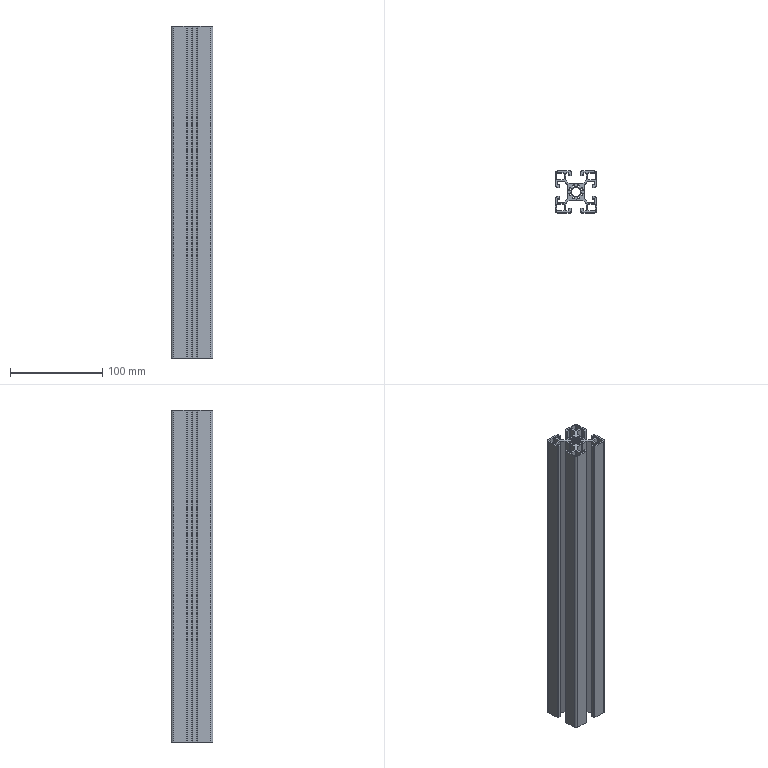Part | STEP file | PN_0029 | 1 solid | 271 faces | box 45 x 45 x 360 mm | volume 230982 mm3 | cylinder 149 | plane 122 | commonest cylinder face diameters 0.6 x48 1 x40 2 x28 10.2 x9 0.4 x8 16 x8